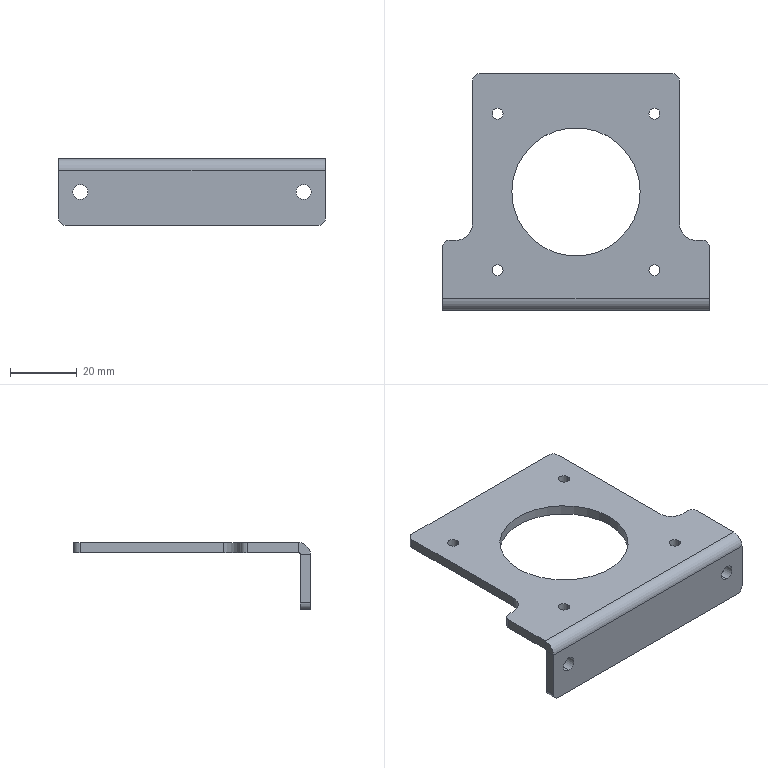Part | STEP file | 1 solid | 40 faces | box 80 x 71 x 20 mm | volume 14540 mm3 | cylinder 24 | plane 16 | commonest cylinder face diameters 3.3 x8 4 x6 4.5 x4 10 x2 38.5 x2 1 x1